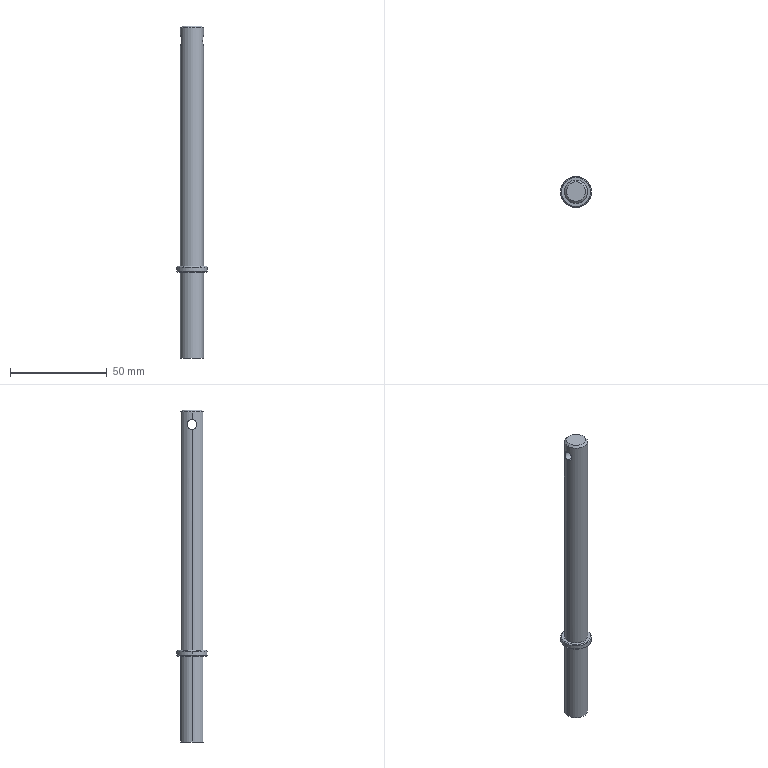Part | STEP file | fBY012F01M-03-01A | 1 solid | 31 faces | box 16 x 16 x 172 mm | volume 18180 mm3 | plane 17 | cylinder 8 | cone 6 | commonest cylinder face diameters 12 x4 5 x2 16 x2